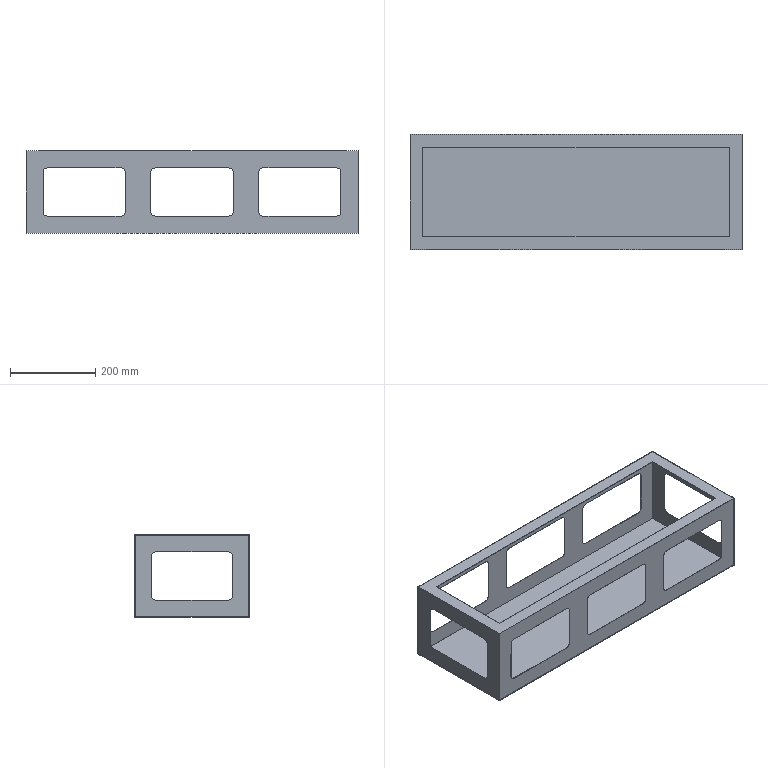Part | SolidWorks | features BaseBody 1 | 1 solid | 80 faces | box 780 x 270 x 193 mm | volume 595214 mm3 | plane 48 | cylinder 32 | commonest cylinder face diameters 20 x32